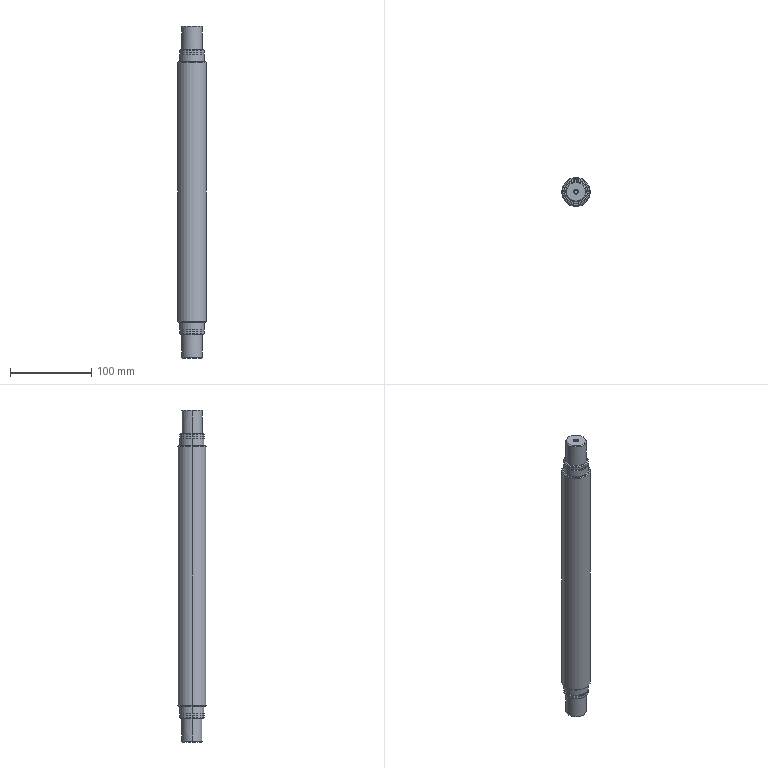Part | STEP file | Idler roller shaft | 1 solid | 50 faces | box 35 x 35 x 408 mm | volume 356727 mm3 | cylinder 22 | cone 16 | plane 12 | commonest cylinder face diameters 30 x8 4 x4 25 x4 28.6 x4 35 x2
STEP:
#1=CARTESIAN_POINT('',(-17.5,0.,334.));
#2=VERTEX_POINT('',#1);
#3=CARTESIAN_POINT('',(17.5,0.,334.));
#4=VERTEX_POINT('',#3);
#5=CARTESIAN_POINT('',(0.,0.,334.));
#6=DIRECTION('',(0.,0.,-1.));
#7=DIRECTION('',(-1.,0.,0.));
#8=AXIS2_PLACEMENT_3D('',#5,#6,#7);
#9=CIRCLE('',#8,17.5);
#10=EDGE_CURVE('',#2,#4,#9,.T.);
#11=ORIENTED_EDGE('',*,*,#10,.T.);
#12=CARTESIAN_POINT('',(17.5,0.,16.));
#13=VERTEX_POINT('',#12);
#14=CARTESIAN_POINT('',(17.5,0.,350.));
#15=DIRECTION('',(0.,0.,-1.));
#16=VECTOR('',#15,1000.);
#17=LINE('',#14,#16);
#18=EDGE_CURVE('',#4,#13,#17,.T.);
#19=ORIENTED_EDGE('',*,*,#18,.T.);
#20=CARTESIAN_POINT('',(-17.5,0.,16.));
#21=VERTEX_POINT('',#20);
#22=CARTESIAN_POINT('',(0.,0.,16.));
#23=DIRECTION('',(0.,0.,1.));
#24=DIRECTION('',(-1.,0.,0.));
#25=AXIS2_PLACEMENT_3D('',#22,#23,#24);
#26=CIRCLE('',#25,17.5);
#27=EDGE_CURVE('',#13,#21,#26,.T.);
#28=ORIENTED_EDGE('',*,*,#27,.T.);
#29=CARTESIAN_POINT('',(-17.5,0.,350.));
#30=DIRECTION('',(0.,0.,-1.));
#31=VECTOR('',#30,1000.);
#32=LINE('',#29,#31);
#33=EDGE_CURVE('',#2,#21,#32,.T.);
#34=ORIENTED_EDGE('',*,*,#33,.F.);
#35=EDGE_LOOP('',(#11,#19,#28,#34));
#36=FACE_OUTER_BOUND('',#35,.T.);
#37=CARTESIAN_POINT('',(0.,0.,350.));
#38=DIRECTION('',(0.,0.,-1.));
#39=DIRECTION('',(-1.,0.,0.));
#40=AXIS2_PLACEMENT_3D('',#37,#38,#39);
#41=CYLINDRICAL_SURFACE('',#40,17.5);
#42=ADVANCED_FACE('',(#36),#41,.T.);
#43=CARTESIAN_POINT('',(16.5,0.,15.));
#44=VERTEX_POINT('',#43);
#45=CARTESIAN_POINT('',(-16.5,0.,15.));
#46=VERTEX_POINT('',#45);
#47=CARTESIAN_POINT('',(0.,0.,15.));
#48=DIRECTION('',(0.,0.,1.));
#49=DIRECTION('',(1.,0.,0.));
#50=AXIS2_PLACEMENT_3D('',#47,#48,#49);
#51=CIRCLE('',#50,16.5);
#52=EDGE_CURVE('',#44,#46,#51,.T.);
#53=ORIENTED_EDGE('',*,*,#52,.T.);
#54=CARTESIAN_POINT('',(-17.5,0.,16.));
#55=DIRECTION('',(-0.7071,0.,0.7071));
#56=VECTOR('',#55,1000.);
#57=LINE('',#54,#56);
#58=EDGE_CURVE('',#46,#21,#57,.T.);
#59=ORIENTED_EDGE('',*,*,#58,.T.);
#60=ORIENTED_EDGE('',*,*,#27,.F.);
#61=CARTESIAN_POINT('',(17.5,0.,16.));
#62=DIRECTION('',(0.7071,0.,0.7071));
#63=VECTOR('',#62,1000.);
#64=LINE('',#61,#63);
#65=EDGE_CURVE('',#44,#13,#64,.T.);
#66=ORIENTED_EDGE('',*,*,#65,.F.);
#67=EDGE_LOOP('',(#53,#59,#60,#66));
#68=FACE_OUTER_BOUND('',#67,.T.);
#69=CARTESIAN_POINT('',(0.,0.,16.));
#70=DIRECTION('',(0.,0.,1.));
#71=DIRECTION('',(1.,0.,0.));
#72=AXIS2_PLACEMENT_3D('',#69,#70,#71);
#73=CONICAL_SURFACE('',#72,17.5,0.7854);
#74=ADVANCED_FACE('',(#68),#73,.T.);
#75=CARTESIAN_POINT('',(-16.5,0.,335.));
#76=VERTEX_POINT('',#75);
#77=CARTESIAN_POINT('',(16.5,0.,335.));
#78=VERTEX_POINT('',#77);
#79=CARTESIAN_POINT('',(0.,0.,335.));
#80=DIRECTION('',(0.,0.,-1.));
#81=DIRECTION('',(-1.,0.,0.));
#82=AXIS2_PLACEMENT_3D('',#79,#80,#81);
#83=CIRCLE('',#82,16.5);
#84=EDGE_CURVE('',#76,#78,#83,.T.);
#85=ORIENTED_EDGE('',*,*,#84,.T.);
#86=CARTESIAN_POINT('',(17.5,0.,334.));
#87=DIRECTION('',(0.7071,0.,-0.7071));
#88=VECTOR('',#87,1000.);
#89=LINE('',#86,#88);
#90=EDGE_CURVE('',#78,#4,#89,.T.);
#91=ORIENTED_EDGE('',*,*,#90,.T.);
#92=ORIENTED_EDGE('',*,*,#10,.F.);
#93=CARTESIAN_POINT('',(-17.5,0.,334.));
#94=DIRECTION('',(-0.7071,0.,-0.7071));
#95=VECTOR('',#94,1000.);
#96=LINE('',#93,#95);
#97=EDGE_CURVE('',#76,#2,#96,.T.);
#98=ORIENTED_EDGE('',*,*,#97,.F.);
#99=EDGE_LOOP('',(#85,#91,#92,#98));
#100=FACE_OUTER_BOUND('',#99,.T.);
#101=CARTESIAN_POINT('',(0.,0.,334.));
#102=DIRECTION('',(0.,0.,-1.));
#103=DIRECTION('',(-1.,0.,0.));
#104=AXIS2_PLACEMENT_3D('',#101,#102,#103);
#105=CONICAL_SURFACE('',#104,17.5,0.7854);
#106=ADVANCED_FACE('',(#100),#105,.T.);
#107=CARTESIAN_POINT('',(15.,0.,15.));
#108=VERTEX_POINT('',#107);
#109=CARTESIAN_POINT('',(-15.,0.,15.));
#110=VERTEX_POINT('',#109);
#111=CARTESIAN_POINT('',(0.,0.,15.));
#112=DIRECTION('',(0.,0.,1.));
#113=DIRECTION('',(-1.,0.,0.));
#114=AXIS2_PLACEMENT_3D('',#111,#112,#113);
#115=CIRCLE('',#114,15.);
#116=EDGE_CURVE('',#108,#110,#115,.T.);
#117=ORIENTED_EDGE('',*,*,#116,.F.);
#118=CARTESIAN_POINT('',(15.,0.,6.));
#119=VERTEX_POINT('',#118);
#120=CARTESIAN_POINT('',(15.,0.,15.));
#121=DIRECTION('',(0.,0.,-1.));
#122=VECTOR('',#121,1000.);
#123=LINE('',#120,#122);
#124=EDGE_CURVE('',#108,#119,#123,.T.);
#125=ORIENTED_EDGE('',*,*,#124,.T.);
#126=CARTESIAN_POINT('',(-15.,0.,6.));
#127=VERTEX_POINT('',#126);
#128=CARTESIAN_POINT('',(0.,0.,6.));
#129=DIRECTION('',(0.,0.,1.));
#130=DIRECTION('',(-1.,0.,0.));
#131=AXIS2_PLACEMENT_3D('',#128,#129,#130);
#132=CIRCLE('',#131,15.);
#133=EDGE_CURVE('',#119,#127,#132,.T.);
#134=ORIENTED_EDGE('',*,*,#133,.T.);
#135=CARTESIAN_POINT('',(-15.,0.,15.));
#136=DIRECTION('',(0.,0.,-1.));
#137=VECTOR('',#136,1000.);
#138=LINE('',#135,#137);
#139=EDGE_CURVE('',#110,#127,#138,.T.);
#140=ORIENTED_EDGE('',*,*,#139,.F.);
#141=EDGE_LOOP('',(#117,#125,#134,#140));
#142=FACE_OUTER_BOUND('',#141,.T.);
#143=CARTESIAN_POINT('',(0.,0.,15.));
#144=DIRECTION('',(0.,0.,-1.));
#145=DIRECTION('',(-1.,0.,0.));
#146=AXIS2_PLACEMENT_3D('',#143,#144,#145);
#147=CYLINDRICAL_SURFACE('',#146,15.);
#148=ADVANCED_FACE('',(#142),#147,.T.);
#149=CARTESIAN_POINT('',(-15.,0.,335.));
#150=VERTEX_POINT('',#149);
#151=CARTESIAN_POINT('',(15.,0.,335.));
#152=VERTEX_POINT('',#151);
#153=CARTESIAN_POINT('',(0.,0.,335.));
#154=DIRECTION('',(0.,0.,-1.));
#155=DIRECTION('',(1.,0.,0.));
#156=AXIS2_PLACEMENT_3D('',#153,#154,#155);
#157=CIRCLE('',#156,15.);
#158=EDGE_CURVE('',#150,#152,#157,.T.);
#159=ORIENTED_EDGE('',*,*,#158,.F.);
#160=CARTESIAN_POINT('',(-15.,0.,344.));
#161=VERTEX_POINT('',#160);
#162=CARTESIAN_POINT('',(-15.,0.,335.));
#163=DIRECTION('',(0.,0.,1.));
#164=VECTOR('',#163,1000.);
#165=LINE('',#162,#164);
#166=EDGE_CURVE('',#150,#161,#165,.T.);
#167=ORIENTED_EDGE('',*,*,#166,.T.);
#168=CARTESIAN_POINT('',(15.,0.,344.));
#169=VERTEX_POINT('',#168);
#170=CARTESIAN_POINT('',(0.,0.,344.));
#171=DIRECTION('',(0.,0.,-1.));
#172=DIRECTION('',(1.,0.,0.));
#173=AXIS2_PLACEMENT_3D('',#170,#171,#172);
#174=CIRCLE('',#173,15.);
#175=EDGE_CURVE('',#161,#169,#174,.T.);
#176=ORIENTED_EDGE('',*,*,#175,.T.);
#177=CARTESIAN_POINT('',(15.,0.,335.));
#178=DIRECTION('',(0.,0.,1.));
#179=VECTOR('',#178,1000.);
#180=LINE('',#177,#179);
#181=EDGE_CURVE('',#152,#169,#180,.T.);
#182=ORIENTED_EDGE('',*,*,#181,.F.);
#183=EDGE_LOOP('',(#159,#167,#176,#182));
#184=FACE_OUTER_BOUND('',#183,.T.);
#185=CARTESIAN_POINT('',(0.,0.,335.));
#186=DIRECTION('',(0.,0.,1.));
#187=DIRECTION('',(1.,0.,0.));
#188=AXIS2_PLACEMENT_3D('',#185,#186,#187);
#189=CYLINDRICAL_SURFACE('',#188,15.);
#190=ADVANCED_FACE('',(#184),#189,.T.);
#191=CARTESIAN_POINT('',(-14.3,0.,6.));
#192=VERTEX_POINT('',#191);
#193=CARTESIAN_POINT('',(14.3,0.,6.));
#194=VERTEX_POINT('',#193);
#195=CARTESIAN_POINT('',(0.,0.,6.));
#196=DIRECTION('',(0.,0.,-1.));
#197=DIRECTION('',(-1.,0.,0.));
#198=AXIS2_PLACEMENT_3D('',#195,#196,#197);
#199=CIRCLE('',#198,14.3);
#200=EDGE_CURVE('',#192,#194,#199,.T.);
#201=ORIENTED_EDGE('',*,*,#200,.T.);
#202=CARTESIAN_POINT('',(14.3,0.,4.));
#203=VERTEX_POINT('',#202);
#204=CARTESIAN_POINT('',(14.3,0.,-29.));
#205=DIRECTION('',(0.,0.,-1.));
#206=VECTOR('',#205,1000.);
#207=LINE('',#204,#206);
#208=EDGE_CURVE('',#194,#203,#207,.T.);
#209=ORIENTED_EDGE('',*,*,#208,.T.);
#210=CARTESIAN_POINT('',(-14.3,0.,4.));
#211=VERTEX_POINT('',#210);
#212=CARTESIAN_POINT('',(0.,0.,4.));
#213=DIRECTION('',(0.,0.,1.));
#214=DIRECTION('',(-1.,0.,0.));
#215=AXIS2_PLACEMENT_3D('',#212,#213,#214);
#216=CIRCLE('',#215,14.3);
#217=EDGE_CURVE('',#203,#211,#216,.T.);
#218=ORIENTED_EDGE('',*,*,#217,.T.);
#219=CARTESIAN_POINT('',(-14.3,0.,-29.));
#220=DIRECTION('',(0.,0.,-1.));
#221=VECTOR('',#220,1000.);
#222=LINE('',#219,#221);
#223=EDGE_CURVE('',#192,#211,#222,.T.);
#224=ORIENTED_EDGE('',*,*,#223,.F.);
#225=EDGE_LOOP('',(#201,#209,#218,#224));
#226=FACE_OUTER_BOUND('',#225,.T.);
#227=CARTESIAN_POINT('',(0.,0.,-29.));
#228=DIRECTION('',(0.,0.,-1.));
#229=DIRECTION('',(-1.,0.,0.));
#230=AXIS2_PLACEMENT_3D('',#227,#228,#229);
#231=CYLINDRICAL_SURFACE('',#230,14.3);
#232=ADVANCED_FACE('',(#226),#231,.T.);
#233=CARTESIAN_POINT('',(-14.3,0.,346.));
#234=VERTEX_POINT('',#233);
#235=CARTESIAN_POINT('',(14.3,0.,346.));
#236=VERTEX_POINT('',#235);
#237=CARTESIAN_POINT('',(0.,0.,346.));
#238=DIRECTION('',(0.,0.,-1.));
#239=DIRECTION('',(-1.,0.,0.));
#240=AXIS2_PLACEMENT_3D('',#237,#238,#239);
#241=CIRCLE('',#240,14.3);
#242=EDGE_CURVE('',#234,#236,#241,.T.);
#243=ORIENTED_EDGE('',*,*,#242,.T.);
#244=CARTESIAN_POINT('',(14.3,0.,344.));
#245=VERTEX_POINT('',#244);
#246=CARTESIAN_POINT('',(14.3,0.,-29.));
#247=DIRECTION('',(0.,0.,-1.));
#248=VECTOR('',#247,1000.);
#249=LINE('',#246,#248);
#250=EDGE_CURVE('',#236,#245,#249,.T.);
#251=ORIENTED_EDGE('',*,*,#250,.T.);
#252=CARTESIAN_POINT('',(-14.3,0.,344.));
#253=VERTEX_POINT('',#252);
#254=CARTESIAN_POINT('',(0.,0.,344.));
#255=DIRECTION('',(0.,0.,1.));
#256=DIRECTION('',(-1.,0.,0.));
#257=AXIS2_PLACEMENT_3D('',#254,#255,#256);
#258=CIRCLE('',#257,14.3);
#259=EDGE_CURVE('',#245,#253,#258,.T.);
#260=ORIENTED_EDGE('',*,*,#259,.T.);
#261=CARTESIAN_POINT('',(-14.3,0.,-29.));
#262=DIRECTION('',(0.,0.,-1.));
#263=VECTOR('',#262,1000.);
#264=LINE('',#261,#263);
#265=EDGE_CURVE('',#234,#253,#264,.T.);
#266=ORIENTED_EDGE('',*,*,#265,.F.);
#267=EDGE_LOOP('',(#243,#251,#260,#266));
#268=FACE_OUTER_BOUND('',#267,.T.);
#269=CARTESIAN_POINT('',(0.,0.,-29.));
#270=DIRECTION('',(0.,0.,-1.));
#271=DIRECTION('',(-1.,0.,0.));
#272=AXIS2_PLACEMENT_3D('',#269,#270,#271);
#273=CYLINDRICAL_SURFACE('',#272,14.3);
#274=ADVANCED_FACE('',(#268),#273,.T.);
#275=CARTESIAN_POINT('',(-15.,0.,4.));
#276=VERTEX_POINT('',#275);
#277=CARTESIAN_POINT('',(15.,0.,4.));
#278=VERTEX_POINT('',#277);
#279=CARTESIAN_POINT('',(0.,0.,4.));
#280=DIRECTION('',(0.,0.,-1.));
#281=DIRECTION('',(-1.,0.,0.));
#282=AXIS2_PLACEMENT_3D('',#279,#280,#281);
#283=CIRCLE('',#282,15.);
#284=EDGE_CURVE('',#276,#278,#283,.T.);
#285=ORIENTED_EDGE('',*,*,#284,.T.);
#286=CARTESIAN_POINT('',(15.,0.,1.));
#287=VERTEX_POINT('',#286);
#288=CARTESIAN_POINT('',(15.,0.,15.));
#289=DIRECTION('',(0.,0.,-1.));
#290=VECTOR('',#289,1000.);
#291=LINE('',#288,#290);
#292=EDGE_CURVE('',#278,#287,#291,.T.);
#293=ORIENTED_EDGE('',*,*,#292,.T.);
#294=CARTESIAN_POINT('',(-15.,0.,1.));
#295=VERTEX_POINT('',#294);
#296=CARTESIAN_POINT('',(0.,0.,1.));
#297=DIRECTION('',(0.,0.,1.));
#298=DIRECTION('',(-1.,0.,0.));
#299=AXIS2_PLACEMENT_3D('',#296,#297,#298);
#300=CIRCLE('',#299,15.);
#301=EDGE_CURVE('',#287,#295,#300,.T.);
#302=ORIENTED_EDGE('',*,*,#301,.T.);
#303=CARTESIAN_POINT('',(-15.,0.,15.));
#304=DIRECTION('',(0.,0.,-1.));
#305=VECTOR('',#304,1000.);
#306=LINE('',#303,#305);
#307=EDGE_CURVE('',#276,#295,#306,.T.);
#308=ORIENTED_EDGE('',*,*,#307,.F.);
#309=EDGE_LOOP('',(#285,#293,#302,#308));
#310=FACE_OUTER_BOUND('',#309,.T.);
#311=CARTESIAN_POINT('',(0.,0.,15.));
#312=DIRECTION('',(0.,0.,-1.));
#313=DIRECTION('',(-1.,0.,0.));
#314=AXIS2_PLACEMENT_3D('',#311,#312,#313);
#315=CYLINDRICAL_SURFACE('',#314,15.);
#316=ADVANCED_FACE('',(#310),#315,.T.);
#317=CARTESIAN_POINT('',(15.,0.,346.));
#318=VERTEX_POINT('',#317);
#319=CARTESIAN_POINT('',(-15.,0.,346.));
#320=VERTEX_POINT('',#319);
#321=CARTESIAN_POINT('',(0.,0.,346.));
#322=DIRECTION('',(0.,0.,1.));
#323=DIRECTION('',(1.,0.,0.));
#324=AXIS2_PLACEMENT_3D('',#321,#322,#323);
#325=CIRCLE('',#324,15.);
#326=EDGE_CURVE('',#318,#320,#325,.T.);
#327=ORIENTED_EDGE('',*,*,#326,.T.);
#328=CARTESIAN_POINT('',(-15.,0.,349.));
#329=VERTEX_POINT('',#328);
#330=CARTESIAN_POINT('',(-15.,0.,335.));
#331=DIRECTION('',(0.,0.,1.));
#332=VECTOR('',#331,1000.);
#333=LINE('',#330,#332);
#334=EDGE_CURVE('',#320,#329,#333,.T.);
#335=ORIENTED_EDGE('',*,*,#334,.T.);
#336=CARTESIAN_POINT('',(15.,0.,349.));
#337=VERTEX_POINT('',#336);
#338=CARTESIAN_POINT('',(0.,0.,349.));
#339=DIRECTION('',(0.,0.,-1.));
#340=DIRECTION('',(1.,0.,0.));
#341=AXIS2_PLACEMENT_3D('',#338,#339,#340);
#342=CIRCLE('',#341,15.);
#343=EDGE_CURVE('',#329,#337,#342,.T.);
#344=ORIENTED_EDGE('',*,*,#343,.T.);
#345=CARTESIAN_POINT('',(15.,0.,335.));
#346=DIRECTION('',(0.,0.,1.));
#347=VECTOR('',#346,1000.);
#348=LINE('',#345,#347);
#349=EDGE_CURVE('',#318,#337,#348,.T.);
#350=ORIENTED_EDGE('',*,*,#349,.F.);
#351=EDGE_LOOP('',(#327,#335,#344,#350));
#352=FACE_OUTER_BOUND('',#351,.T.);
#353=CARTESIAN_POINT('',(0.,0.,335.));
#354=DIRECTION('',(0.,0.,1.));
#355=DIRECTION('',(1.,0.,0.));
#356=AXIS2_PLACEMENT_3D('',#353,#354,#355);
#357=CYLINDRICAL_SURFACE('',#356,15.);
#358=ADVANCED_FACE('',(#352),#357,.T.);
#359=CARTESIAN_POINT('',(14.,0.,0.));
#360=VERTEX_POINT('',#359);
#361=CARTESIAN_POINT('',(-14.,0.,0.));
#362=VERTEX_POINT('',#361);
#363=CARTESIAN_POINT('',(0.,0.,0.));
#364=DIRECTION('',(0.,0.,1.));
#365=DIRECTION('',(1.,0.,0.));
#366=AXIS2_PLACEMENT_3D('',#363,#364,#365);
#367=CIRCLE('',#366,14.);
#368=EDGE_CURVE('',#360,#362,#367,.T.);
#369=ORIENTED_EDGE('',*,*,#368,.T.);
#370=CARTESIAN_POINT('',(-15.,0.,1.));
#371=DIRECTION('',(-0.7071,0.,0.7071));
#372=VECTOR('',#371,1000.);
#373=LINE('',#370,#372);
#374=EDGE_CURVE('',#362,#295,#373,.T.);
#375=ORIENTED_EDGE('',*,*,#374,.T.);
#376=ORIENTED_EDGE('',*,*,#301,.F.);
#377=CARTESIAN_POINT('',(15.,0.,1.));
#378=DIRECTION('',(0.7071,0.,0.7071));
#379=VECTOR('',#378,1000.);
#380=LINE('',#377,#379);
#381=EDGE_CURVE('',#360,#287,#380,.T.);
#382=ORIENTED_EDGE('',*,*,#381,.F.);
#383=EDGE_LOOP('',(#369,#375,#376,#382));
#384=FACE_OUTER_BOUND('',#383,.T.);
#385=CARTESIAN_POINT('',(0.,0.,1.));
#386=DIRECTION('',(0.,0.,1.));
#387=DIRECTION('',(1.,0.,0.));
#388=AXIS2_PLACEMENT_3D('',#385,#386,#387);
#389=CONICAL_SURFACE('',#388,15.,0.7854);
#390=ADVANCED_FACE('',(#384),#389,.T.);
#391=CARTESIAN_POINT('',(-14.,0.,350.));
#392=VERTEX_POINT('',#391);
#393=CARTESIAN_POINT('',(14.,0.,350.));
#394=VERTEX_POINT('',#393);
#395=CARTESIAN_POINT('',(0.,0.,350.));
#396=DIRECTION('',(0.,0.,-1.));
#397=DIRECTION('',(-1.,0.,0.));
#398=AXIS2_PLACEMENT_3D('',#395,#396,#397);
#399=CIRCLE('',#398,14.);
#400=EDGE_CURVE('',#392,#394,#399,.T.);
#401=ORIENTED_EDGE('',*,*,#400,.T.);
#402=CARTESIAN_POINT('',(15.,0.,349.));
#403=DIRECTION('',(0.7071,0.,-0.7071));
#404=VECTOR('',#403,1000.);
#405=LINE('',#402,#404);
#406=EDGE_CURVE('',#394,#337,#405,.T.);
#407=ORIENTED_EDGE('',*,*,#406,.T.);
#408=ORIENTED_EDGE('',*,*,#343,.F.);
#409=CARTESIAN_POINT('',(-15.,0.,349.));
#410=DIRECTION('',(-0.7071,0.,-0.7071));
#411=VECTOR('',#410,1000.);
#412=LINE('',#409,#411);
#413=EDGE_CURVE('',#392,#329,#412,.T.);
#414=ORIENTED_EDGE('',*,*,#413,.F.);
#415=EDGE_LOOP('',(#401,#407,#408,#414));
#416=FACE_OUTER_BOUND('',#415,.T.);
#417=CARTESIAN_POINT('',(0.,0.,349.));
#418=DIRECTION('',(0.,0.,-1.));
#419=DIRECTION('',(-1.,0.,0.));
#420=AXIS2_PLACEMENT_3D('',#417,#418,#419);
#421=CONICAL_SURFACE('',#420,15.,0.7854);
#422=ADVANCED_FACE('',(#416),#421,.T.);
#423=CARTESIAN_POINT('',(0.,12.5,-28.));
#424=VERTEX_POINT('',#423);
#425=CARTESIAN_POINT('',(-12.5,0.,-28.));
#426=VERTEX_POINT('',#425);
#427=CARTESIAN_POINT('',(0.,0.,-28.));
#428=DIRECTION('',(0.,0.,1.));
#429=DIRECTION('',(1.,0.,0.));
#430=AXIS2_PLACEMENT_3D('',#427,#428,#429);
#431=CIRCLE('',#430,12.5);
#432=EDGE_CURVE('',#424,#426,#431,.T.);
#433=ORIENTED_EDGE('',*,*,#432,.T.);
#434=CARTESIAN_POINT('',(-12.5,0.,0.));
#435=VERTEX_POINT('',#434);
#436=CARTESIAN_POINT('',(-12.5,0.,-29.));
#437=DIRECTION('',(0.,0.,1.));
#438=VECTOR('',#437,1000.);
#439=LINE('',#436,#438);
#440=EDGE_CURVE('',#426,#435,#439,.T.);
#441=ORIENTED_EDGE('',*,*,#440,.T.);
#442=CARTESIAN_POINT('',(12.5,0.,0.));
#443=VERTEX_POINT('',#442);
#444=CARTESIAN_POINT('',(0.,0.,0.));
#445=DIRECTION('',(0.,0.,-1.));
#446=DIRECTION('',(1.,0.,0.));
#447=AXIS2_PLACEMENT_3D('',#444,#445,#446);
#448=CIRCLE('',#447,12.5);
#449=EDGE_CURVE('',#435,#443,#448,.T.);
#450=ORIENTED_EDGE('',*,*,#449,.T.);
#451=CARTESIAN_POINT('',(12.5,0.,-28.));
#452=VERTEX_POINT('',#451);
#453=CARTESIAN_POINT('',(12.5,0.,-29.));
#454=DIRECTION('',(0.,0.,1.));
#455=VECTOR('',#454,1000.);
#456=LINE('',#453,#455);
#457=EDGE_CURVE('',#452,#443,#456,.T.);
#458=ORIENTED_EDGE('',*,*,#457,.F.);
#459=CARTESIAN_POINT('',(0.,0.,-28.));
#460=DIRECTION('',(0.,0.,1.));
#461=DIRECTION('',(1.,0.,0.));
#462=AXIS2_PLACEMENT_3D('',#459,#460,#461);
#463=CIRCLE('',#462,12.5);
#464=EDGE_CURVE('',#452,#424,#463,.T.);
#465=ORIENTED_EDGE('',*,*,#464,.T.);
#466=EDGE_LOOP('',(#433,#441,#450,#458,#465));
#467=FACE_OUTER_BOUND('',#466,.T.);
#468=CARTESIAN_POINT('',(0.,0.,-29.));
#469=DIRECTION('',(0.,0.,1.));
#470=DIRECTION('',(1.,0.,0.));
#471=AXIS2_PLACEMENT_3D('',#468,#469,#470);
#472=CYLINDRICAL_SURFACE('',#471,12.5);
#473=ADVANCED_FACE('',(#467),#472,.T.);
#474=CARTESIAN_POINT('',(0.,12.5,378.));
#475=VERTEX_POINT('',#474);
#476=CARTESIAN_POINT('',(12.5,0.,378.));
#477=VERTEX_POINT('',#476);
#478=CARTESIAN_POINT('',(0.,0.,378.));
#479=DIRECTION('',(0.,0.,-1.));
#480=DIRECTION('',(-1.,0.,0.));
#481=AXIS2_PLACEMENT_3D('',#478,#479,#480);
#482=CIRCLE('',#481,12.5);
#483=EDGE_CURVE('',#475,#477,#482,.T.);
#484=ORIENTED_EDGE('',*,*,#483,.T.);
#485=CARTESIAN_POINT('',(12.5,0.,350.));
#486=VERTEX_POINT('',#485);
#487=CARTESIAN_POINT('',(12.5,0.,379.));
#488=DIRECTION('',(0.,0.,-1.));
#489=VECTOR('',#488,1000.);
#490=LINE('',#487,#489);
#491=EDGE_CURVE('',#477,#486,#490,.T.);
#492=ORIENTED_EDGE('',*,*,#491,.T.);
#493=CARTESIAN_POINT('',(-12.5,0.,350.));
#494=VERTEX_POINT('',#493);
#495=CARTESIAN_POINT('',(0.,0.,350.));
#496=DIRECTION('',(0.,0.,-1.));
#497=DIRECTION('',(-1.,0.,0.));
#498=AXIS2_PLACEMENT_3D('',#495,#496,#497);
#499=CIRCLE('',#498,12.5);
#500=EDGE_CURVE('',#494,#486,#499,.T.);
#501=ORIENTED_EDGE('',*,*,#500,.F.);
#502=CARTESIAN_POINT('',(-12.5,0.,378.));
#503=VERTEX_POINT('',#502);
#504=CARTESIAN_POINT('',(-12.5,0.,379.));
#505=DIRECTION('',(0.,0.,-1.));
#506=VECTOR('',#505,1000.);
#507=LINE('',#504,#506);
#508=EDGE_CURVE('',#503,#494,#507,.T.);
#509=ORIENTED_EDGE('',*,*,#508,.F.);
#510=CARTESIAN_POINT('',(0.,0.,378.));
#511=DIRECTION('',(0.,0.,-1.));
#512=DIRECTION('',(-1.,0.,0.));
#513=AXIS2_PLACEMENT_3D('',#510,#511,#512);
#514=CIRCLE('',#513,12.5);
#515=EDGE_CURVE('',#503,#475,#514,.T.);
#516=ORIENTED_EDGE('',*,*,#515,.T.);
#517=EDGE_LOOP('',(#484,#492,#501,#509,#516));
#518=FACE_OUTER_BOUND('',#517,.T.);
#519=CARTESIAN_POINT('',(0.,0.,379.));
#520=DIRECTION('',(0.,0.,-1.));
#521=DIRECTION('',(-1.,0.,0.));
#522=AXIS2_PLACEMENT_3D('',#519,#520,#521);
#523=CYLINDRICAL_SURFACE('',#522,12.5);
#524=ADVANCED_FACE('',(#518),#523,.T.);
#525=CARTESIAN_POINT('',(0.,-11.5,-29.));
#526=VERTEX_POINT('',#525);
#527=CARTESIAN_POINT('',(0.,11.5,-29.));
#528=VERTEX_POINT('',#527);
#529=CARTESIAN_POINT('',(0.,0.,-29.));
#530=DIRECTION('',(0.,0.,1.));
#531=DIRECTION('',(0.,-1.,0.));
#532=AXIS2_PLACEMENT_3D('',#529,#530,#531);
#533=CIRCLE('',#532,11.5);
#534=EDGE_CURVE('',#526,#528,#533,.T.);
#535=ORIENTED_EDGE('',*,*,#534,.T.);
#536=CARTESIAN_POINT('',(0.,12.5,-28.));
#537=DIRECTION('',(0.,0.7071,0.7071));
#538=VECTOR('',#537,1000.);
#539=LINE('',#536,#538);
#540=EDGE_CURVE('',#528,#424,#539,.T.);
#541=ORIENTED_EDGE('',*,*,#540,.T.);
#542=ORIENTED_EDGE('',*,*,#464,.F.);
#543=CARTESIAN_POINT('',(0.,-12.5,-28.));
#544=VERTEX_POINT('',#543);
#545=CARTESIAN_POINT('',(0.,0.,-28.));
#546=DIRECTION('',(0.,0.,1.));
#547=DIRECTION('',(1.,0.,0.));
#548=AXIS2_PLACEMENT_3D('',#545,#546,#547);
#549=CIRCLE('',#548,12.5);
#550=EDGE_CURVE('',#544,#452,#549,.T.);
#551=ORIENTED_EDGE('',*,*,#550,.F.);
#552=CARTESIAN_POINT('',(0.,-12.5,-28.));
#553=DIRECTION('',(0.,-0.7071,0.7071));
#554=VECTOR('',#553,1000.);
#555=LINE('',#552,#554);
#556=EDGE_CURVE('',#526,#544,#555,.T.);
#557=ORIENTED_EDGE('',*,*,#556,.F.);
#558=EDGE_LOOP('',(#535,#541,#542,#551,#557));
#559=FACE_OUTER_BOUND('',#558,.T.);
#560=CARTESIAN_POINT('',(0.,0.,-28.));
#561=DIRECTION('',(0.,0.,1.));
#562=DIRECTION('',(0.,-1.,0.));
#563=AXIS2_PLACEMENT_3D('',#560,#561,#562);
#564=CONICAL_SURFACE('',#563,12.5,0.7854);
#565=ADVANCED_FACE('',(#559),#564,.T.);
#566=CARTESIAN_POINT('',(0.,11.5,379.));
#567=VERTEX_POINT('',#566);
#568=CARTESIAN_POINT('',(0.,-11.5,379.));
#569=VERTEX_POINT('',#568);
#570=CARTESIAN_POINT('',(0.,0.,379.));
#571=DIRECTION('',(0.,0.,-1.));
#572=DIRECTION('',(0.,1.,0.));
#573=AXIS2_PLACEMENT_3D('',#570,#571,#572);
#574=CIRCLE('',#573,11.5);
#575=EDGE_CURVE('',#567,#569,#574,.T.);
#576=ORIENTED_EDGE('',*,*,#575,.T.);
#577=CARTESIAN_POINT('',(0.,-12.5,378.));
#578=VERTEX_POINT('',#577);
#579=CARTESIAN_POINT('',(0.,-12.5,378.));
#580=DIRECTION('',(0.,-0.7071,-0.7071));
#581=VECTOR('',#580,1000.);
#582=LINE('',#579,#581);
#583=EDGE_CURVE('',#569,#578,#582,.T.);
#584=ORIENTED_EDGE('',*,*,#583,.T.);
#585=CARTESIAN_POINT('',(0.,0.,378.));
#586=DIRECTION('',(0.,0.,-1.));
#587=DIRECTION('',(-1.,0.,0.));
#588=AXIS2_PLACEMENT_3D('',#585,#586,#587);
#589=CIRCLE('',#588,12.5);
#590=EDGE_CURVE('',#477,#578,#589,.T.);
#591=ORIENTED_EDGE('',*,*,#590,.F.);
#592=ORIENTED_EDGE('',*,*,#483,.F.);
#593=CARTESIAN_POINT('',(0.,12.5,378.));
#594=DIRECTION('',(0.,0.7071,-0.7071));
#595=VECTOR('',#594,1000.);
#596=LINE('',#593,#595);
#597=EDGE_CURVE('',#567,#475,#596,.T.);
#598=ORIENTED_EDGE('',*,*,#597,.F.);
#599=EDGE_LOOP('',(#576,#584,#591,#592,#598));
#600=FACE_OUTER_BOUND('',#599,.T.);
#601=CARTESIAN_POINT('',(0.,0.,378.));
#602=DIRECTION('',(0.,0.,-1.));
#603=DIRECTION('',(0.,1.,0.));
#604=AXIS2_PLACEMENT_3D('',#601,#602,#603);
#605=CONICAL_SURFACE('',#604,12.5,0.7854);
#606=ADVANCED_FACE('',(#600),#605,.T.);
#607=CARTESIAN_POINT('',(0.,-2.,-28.));
#608=VERTEX_POINT('',#607);
#609=CARTESIAN_POINT('',(-2.,0.,-28.));
#610=VERTEX_POINT('',#609);
#611=CARTESIAN_POINT('',(0.,0.,-28.));
#612=DIRECTION('',(0.,0.,-1.));
#613=DIRECTION('',(-1.,0.,0.));
#614=AXIS2_PLACEMENT_3D('',#611,#612,#613);
#615=CIRCLE('',#614,2.);
#616=EDGE_CURVE('',#608,#610,#615,.T.);
#617=ORIENTED_EDGE('',*,*,#616,.F.);
#618=CARTESIAN_POINT('',(0.,-3.,-29.));
#619=VERTEX_POINT('',#618);
#620=CARTESIAN_POINT('',(0.,-3.,-29.));
#621=DIRECTION('',(0.,-0.7071,-0.7071));
#622=VECTOR('',#621,1000.);
#623=LINE('',#620,#622);
#624=EDGE_CURVE('',#608,#619,#623,.T.);
#625=ORIENTED_EDGE('',*,*,#624,.T.);
#626=CARTESIAN_POINT('',(0.,3.,-29.));
#627=VERTEX_POINT('',#626);
#628=CARTESIAN_POINT('',(0.,0.,-29.));
#629=DIRECTION('',(0.,0.,1.));
#630=DIRECTION('',(0.,1.,0.));
#631=AXIS2_PLACEMENT_3D('',#628,#629,#630);
#632=CIRCLE('',#631,3.);
#633=EDGE_CURVE('',#627,#619,#632,.T.);
#634=ORIENTED_EDGE('',*,*,#633,.F.);
#635=CARTESIAN_POINT('',(0.,2.,-28.));
#636=VERTEX_POINT('',#635);
#637=CARTESIAN_POINT('',(0.,3.,-29.));
#638=DIRECTION('',(0.,0.7071,-0.7071));
#639=VECTOR('',#638,1000.);
#640=LINE('',#637,#639);
#641=EDGE_CURVE('',#636,#627,#640,.T.);
#642=ORIENTED_EDGE('',*,*,#641,.F.);
#643=CARTESIAN_POINT('',(0.,0.,-28.));
#644=DIRECTION('',(0.,0.,-1.));
#645=DIRECTION('',(-1.,0.,0.));
#646=AXIS2_PLACEMENT_3D('',#643,#644,#645);
#647=CIRCLE('',#646,2.);
#648=EDGE_CURVE('',#610,#636,#647,.T.);
#649=ORIENTED_EDGE('',*,*,#648,.F.);
#650=EDGE_LOOP('',(#617,#625,#634,#642,#649));
#651=FACE_OUTER_BOUND('',#650,.T.);
#652=CARTESIAN_POINT('',(0.,0.,-29.));
#653=DIRECTION('',(0.,0.,-1.));
#654=DIRECTION('',(0.,1.,0.));
#655=AXIS2_PLACEMENT_3D('',#652,#653,#654);
#656=CONICAL_SURFACE('',#655,3.,0.7854);
#657=ADVANCED_FACE('',(#651),#656,.F.);
#658=CARTESIAN_POINT('',(-2.,0.,378.));
#659=VERTEX_POINT('',#658);
#660=CARTESIAN_POINT('',(2.,0.,378.));
#661=VERTEX_POINT('',#660);
#662=CARTESIAN_POINT('',(0.,0.,378.));
#663=DIRECTION('',(0.,0.,1.));
#664=DIRECTION('',(1.,0.,0.));
#665=AXIS2_PLACEMENT_3D('',#662,#663,#664);
#666=CIRCLE('',#665,2.);
#667=EDGE_CURVE('',#659,#661,#666,.T.);
#668=ORIENTED_EDGE('',*,*,#667,.F.);
#669=CARTESIAN_POINT('',(-3.,0.,379.));
#670=VERTEX_POINT('',#669);
#671=CARTESIAN_POINT('',(-3.,0.,379.));
#672=DIRECTION('',(-0.7071,0.,0.7071));
#673=VECTOR('',#672,1000.);
#674=LINE('',#671,#673);
#675=EDGE_CURVE('',#659,#670,#674,.T.);
#676=ORIENTED_EDGE('',*,*,#675,.T.);
#677=CARTESIAN_POINT('',(3.,0.,379.));
#678=VERTEX_POINT('',#677);
#679=CARTESIAN_POINT('',(0.,0.,379.));
#680=DIRECTION('',(0.,0.,-1.));
#681=DIRECTION('',(1.,0.,0.));
#682=AXIS2_PLACEMENT_3D('',#679,#680,#681);
#683=CIRCLE('',#682,3.);
#684=EDGE_CURVE('',#678,#670,#683,.T.);
#685=ORIENTED_EDGE('',*,*,#684,.F.);
#686=CARTESIAN_POINT('',(3.,0.,379.));
#687=DIRECTION('',(0.7071,0.,0.7071));
#688=VECTOR('',#687,1000.);
#689=LINE('',#686,#688);
#690=EDGE_CURVE('',#661,#678,#689,.T.);
#691=ORIENTED_EDGE('',*,*,#690,.F.);
#692=EDGE_LOOP('',(#668,#676,#685,#691));
#693=FACE_OUTER_BOUND('',#692,.T.);
#694=CARTESIAN_POINT('',(0.,0.,379.));
#695=DIRECTION('',(0.,0.,1.));
#696=DIRECTION('',(1.,0.,0.));
#697=AXIS2_PLACEMENT_3D('',#694,#695,#696);
#698=CONICAL_SURFACE('',#697,3.,0.7854);
#699=ADVANCED_FACE('',(#693),#698,.F.);
#700=CARTESIAN_POINT('',(2.,0.,-18.));
#701=VERTEX_POINT('',#700);
#702=CARTESIAN_POINT('',(-2.,0.,-18.));
#703=VERTEX_POINT('',#702);
#704=CARTESIAN_POINT('',(0.,0.,-18.));
#705=DIRECTION('',(0.,0.,-1.));
#706=DIRECTION('',(-1.,0.,0.));
#707=AXIS2_PLACEMENT_3D('',#704,#705,#706);
#708=CIRCLE('',#707,2.);
#709=EDGE_CURVE('',#701,#703,#708,.T.);
#710=ORIENTED_EDGE('',*,*,#709,.F.);
#711=CARTESIAN_POINT('',(2.,0.,-28.));
#712=VERTEX_POINT('',#711);
#713=CARTESIAN_POINT('',(2.,0.,-18.));
#714=DIRECTION('',(0.,0.,-1.));
#715=VECTOR('',#714,1000.);
#716=LINE('',#713,#715);
#717=EDGE_CURVE('',#701,#712,#716,.T.);
#718=ORIENTED_EDGE('',*,*,#717,.T.);
#719=CARTESIAN_POINT('',(0.,0.,-28.));
#720=DIRECTION('',(0.,0.,-1.));
#721=DIRECTION('',(-1.,0.,0.));
#722=AXIS2_PLACEMENT_3D('',#719,#720,#721);
#723=CIRCLE('',#722,2.);
#724=EDGE_CURVE('',#712,#608,#723,.T.);
#725=ORIENTED_EDGE('',*,*,#724,.T.);
#726=ORIENTED_EDGE('',*,*,#616,.T.);
#727=CARTESIAN_POINT('',(-2.,0.,-18.));
#728=DIRECTION('',(0.,0.,-1.));
#729=VECTOR('',#728,1000.);
#730=LINE('',#727,#729);
#731=EDGE_CURVE('',#703,#610,#730,.T.);
#732=ORIENTED_EDGE('',*,*,#731,.F.);
#733=EDGE_LOOP('',(#710,#718,#725,#726,#732));
#734=FACE_OUTER_BOUND('',#733,.T.);
#735=CARTESIAN_POINT('',(0.,0.,-18.));
#736=DIRECTION('',(0.,0.,-1.));
#737=DIRECTION('',(-1.,0.,0.));
#738=AXIS2_PLACEMENT_3D('',#735,#736,#737);
#739=CYLINDRICAL_SURFACE('',#738,2.);
#740=ADVANCED_FACE('',(#734),#739,.F.);
#741=CARTESIAN_POINT('',(-2.,0.,368.));
#742=VERTEX_POINT('',#741);
#743=CARTESIAN_POINT('',(2.,0.,368.));
#744=VERTEX_POINT('',#743);
#745=CARTESIAN_POINT('',(0.,0.,368.));
#746=DIRECTION('',(0.,0.,1.));
#747=DIRECTION('',(1.,0.,0.));
#748=AXIS2_PLACEMENT_3D('',#745,#746,#747);
#749=CIRCLE('',#748,2.);
#750=EDGE_CURVE('',#742,#744,#749,.T.);
#751=ORIENTED_EDGE('',*,*,#750,.F.);
#752=CARTESIAN_POINT('',(-2.,0.,368.));
#753=DIRECTION('',(0.,0.,1.));
#754=VECTOR('',#753,1000.);
#755=LINE('',#752,#754);
#756=EDGE_CURVE('',#742,#659,#755,.T.);
#757=ORIENTED_EDGE('',*,*,#756,.T.);
#758=ORIENTED_EDGE('',*,*,#667,.T.);
#759=CARTESIAN_POINT('',(2.,0.,368.));
#760=DIRECTION('',(0.,0.,1.));
#761=VECTOR('',#760,1000.);
#762=LINE('',#759,#761);
#763=EDGE_CURVE('',#744,#661,#762,.T.);
#764=ORIENTED_EDGE('',*,*,#763,.F.);
#765=EDGE_LOOP('',(#751,#757,#758,#764));
#766=FACE_OUTER_BOUND('',#765,.T.);
#767=CARTESIAN_POINT('',(0.,0.,368.));
#768=DIRECTION('',(0.,0.,1.));
#769=DIRECTION('',(1.,0.,0.));
#770=AXIS2_PLACEMENT_3D('',#767,#768,#769);
#771=CYLINDRICAL_SURFACE('',#770,2.);
#772=ADVANCED_FACE('',(#766),#771,.F.);
#773=ORIENTED_EDGE('',*,*,#18,.F.);
#774=CARTESIAN_POINT('',(0.,0.,334.));
#775=DIRECTION('',(0.,0.,-1.));
#776=DIRECTION('',(-1.,0.,0.));
#777=AXIS2_PLACEMENT_3D('',#774,#775,#776);
#778=CIRCLE('',#777,17.5);
#779=EDGE_CURVE('',#4,#2,#778,.T.);
#780=ORIENTED_EDGE('',*,*,#779,.T.);
#781=ORIENTED_EDGE('',*,*,#33,.T.);
#782=CARTESIAN_POINT('',(0.,0.,16.));
#783=DIRECTION('',(0.,0.,1.));
#784=DIRECTION('',(-1.,0.,0.));
#785=AXIS2_PLACEMENT_3D('',#782,#783,#784);
#786=CIRCLE('',#785,17.5);
#787=EDGE_CURVE('',#21,#13,#786,.T.);
#788=ORIENTED_EDGE('',*,*,#787,.T.);
#789=EDGE_LOOP('',(#773,#780,#781,#788));
#790=FACE_OUTER_BOUND('',#789,.T.);
#791=CARTESIAN_POINT('',(0.,0.,350.));
#792=DIRECTION('',(0.,0.,-1.));
#793=DIRECTION('',(-1.,0.,0.));
#794=AXIS2_PLACEMENT_3D('',#791,#792,#793);
#795=CYLINDRICAL_SURFACE('',#794,17.5);
#796=ADVANCED_FACE('',(#790),#795,.T.);
#797=ORIENTED_EDGE('',*,*,#58,.F.);
#798=CARTESIAN_POINT('',(0.,0.,15.));
#799=DIRECTION('',(0.,0.,1.));
#800=DIRECTION('',(1.,0.,0.));
#801=AXIS2_PLACEMENT_3D('',#798,#799,#800);
#802=CIRCLE('',#801,16.5);
#803=EDGE_CURVE('',#46,#44,#802,.T.);
#804=ORIENTED_EDGE('',*,*,#803,.T.);
#805=ORIENTED_EDGE('',*,*,#65,.T.);
#806=ORIENTED_EDGE('',*,*,#787,.F.);
#807=EDGE_LOOP('',(#797,#804,#805,#806));
#808=FACE_OUTER_BOUND('',#807,.T.);
#809=CARTESIAN_POINT('',(0.,0.,16.));
#810=DIRECTION('',(0.,0.,1.));
#811=DIRECTION('',(1.,0.,0.));
#812=AXIS2_PLACEMENT_3D('',#809,#810,#811);
#813=CONICAL_SURFACE('',#812,17.5,0.7854);
#814=ADVANCED_FACE('',(#808),#813,.T.);
#815=ORIENTED_EDGE('',*,*,#90,.F.);
#816=CARTESIAN_POINT('',(0.,0.,335.));
#817=DIRECTION('',(0.,0.,-1.));
#818=DIRECTION('',(-1.,0.,0.));
#819=AXIS2_PLACEMENT_3D('',#816,#817,#818);
#820=CIRCLE('',#819,16.5);
#821=EDGE_CURVE('',#78,#76,#820,.T.);
#822=ORIENTED_EDGE('',*,*,#821,.T.);
#823=ORIENTED_EDGE('',*,*,#97,.T.);
#824=ORIENTED_EDGE('',*,*,#779,.F.);
#825=EDGE_LOOP('',(#815,#822,#823,#824));
#826=FACE_OUTER_BOUND('',#825,.T.);
#827=CARTESIAN_POINT('',(0.,0.,334.));
#828=DIRECTION('',(0.,0.,-1.));
#829=DIRECTION('',(-1.,0.,0.));
#830=AXIS2_PLACEMENT_3D('',#827,#828,#829);
#831=CONICAL_SURFACE('',#830,17.5,0.7854);
#832=ADVANCED_FACE('',(#826),#831,.T.);
#833=CARTESIAN_POINT('',(0.,0.,15.));
#834=DIRECTION('',(0.,0.,1.));
#835=DIRECTION('',(-1.,0.,0.));
#836=AXIS2_PLACEMENT_3D('',#833,#834,#835);
#837=CIRCLE('',#836,15.);
#838=EDGE_CURVE('',#110,#108,#837,.T.);
#839=ORIENTED_EDGE('',*,*,#838,.T.);
#840=ORIENTED_EDGE('',*,*,#116,.T.);
#841=EDGE_LOOP('',(#839,#840));
#842=FACE_BOUND('',#841,.T.);
#843=ORIENTED_EDGE('',*,*,#52,.F.);
#844=ORIENTED_EDGE('',*,*,#803,.F.);
#845=EDGE_LOOP('',(#843,#844));
#846=FACE_OUTER_BOUND('',#845,.T.);
#847=CARTESIAN_POINT('',(0.,0.,15.));
#848=DIRECTION('',(0.,0.,-1.));
#849=DIRECTION('',(-1.,0.,0.));
#850=AXIS2_PLACEMENT_3D('',#847,#848,#849);
#851=PLANE('',#850);
#852=ADVANCED_FACE('',(#842,#846),#851,.T.);
#853=CARTESIAN_POINT('',(0.,0.,335.));
#854=DIRECTION('',(0.,0.,-1.));
#855=DIRECTION('',(1.,0.,0.));
#856=AXIS2_PLACEMENT_3D('',#853,#854,#855);
#857=CIRCLE('',#856,15.);
#858=EDGE_CURVE('',#152,#150,#857,.T.);
#859=ORIENTED_EDGE('',*,*,#858,.T.);
#860=ORIENTED_EDGE('',*,*,#158,.T.);
#861=EDGE_LOOP('',(#859,#860));
#862=FACE_BOUND('',#861,.T.);
#863=ORIENTED_EDGE('',*,*,#84,.F.);
#864=ORIENTED_EDGE('',*,*,#821,.F.);
#865=EDGE_LOOP('',(#863,#864));
#866=FACE_OUTER_BOUND('',#865,.T.);
#867=CARTESIAN_POINT('',(0.,0.,335.));
#868=DIRECTION('',(0.,0.,1.));
#869=DIRECTION('',(1.,0.,0.));
#870=AXIS2_PLACEMENT_3D('',#867,#868,#869);
#871=PLANE('',#870);
#872=ADVANCED_FACE('',(#862,#866),#871,.T.);
#873=ORIENTED_EDGE('',*,*,#124,.F.);
#874=ORIENTED_EDGE('',*,*,#838,.F.);
#875=ORIENTED_EDGE('',*,*,#139,.T.);
#876=CARTESIAN_POINT('',(0.,0.,6.));
#877=DIRECTION('',(0.,0.,1.));
#878=DIRECTION('',(-1.,0.,0.));
#879=AXIS2_PLACEMENT_3D('',#876,#877,#878);
#880=CIRCLE('',#879,15.);
#881=EDGE_CURVE('',#127,#119,#880,.T.);
#882=ORIENTED_EDGE('',*,*,#881,.T.);
#883=EDGE_LOOP('',(#873,#874,#875,#882));
#884=FACE_OUTER_BOUND('',#883,.T.);
#885=CARTESIAN_POINT('',(0.,0.,15.));
#886=DIRECTION('',(0.,0.,-1.));
#887=DIRECTION('',(-1.,0.,0.));
#888=AXIS2_PLACEMENT_3D('',#885,#886,#887);
#889=CYLINDRICAL_SURFACE('',#888,15.);
#890=ADVANCED_FACE('',(#884),#889,.T.);
#891=ORIENTED_EDGE('',*,*,#166,.F.);
#892=ORIENTED_EDGE('',*,*,#858,.F.);
#893=ORIENTED_EDGE('',*,*,#181,.T.);
#894=CARTESIAN_POINT('',(0.,0.,344.));
#895=DIRECTION('',(0.,0.,-1.));
#896=DIRECTION('',(1.,0.,0.));
#897=AXIS2_PLACEMENT_3D('',#894,#895,#896);
#898=CIRCLE('',#897,15.);
#899=EDGE_CURVE('',#169,#161,#898,.T.);
#900=ORIENTED_EDGE('',*,*,#899,.T.);
#901=EDGE_LOOP('',(#891,#892,#893,#900));
#902=FACE_OUTER_BOUND('',#901,.T.);
#903=CARTESIAN_POINT('',(0.,0.,335.));
#904=DIRECTION('',(0.,0.,1.));
#905=DIRECTION('',(1.,0.,0.));
#906=AXIS2_PLACEMENT_3D('',#903,#904,#905);
#907=CYLINDRICAL_SURFACE('',#906,15.);
#908=ADVANCED_FACE('',(#902),#907,.T.);
#909=ORIENTED_EDGE('',*,*,#200,.F.);
#910=CARTESIAN_POINT('',(0.,0.,6.));
#911=DIRECTION('',(0.,0.,-1.));
#912=DIRECTION('',(-1.,0.,0.));
#913=AXIS2_PLACEMENT_3D('',#910,#911,#912);
#914=CIRCLE('',#913,14.3);
#915=EDGE_CURVE('',#194,#192,#914,.T.);
#916=ORIENTED_EDGE('',*,*,#915,.F.);
#917=EDGE_LOOP('',(#909,#916));
#918=FACE_BOUND('',#917,.T.);
#919=ORIENTED_EDGE('',*,*,#881,.F.);
#920=ORIENTED_EDGE('',*,*,#133,.F.);
#921=EDGE_LOOP('',(#919,#920));
#922=FACE_OUTER_BOUND('',#921,.T.);
#923=CARTESIAN_POINT('',(-19.3,0.,6.));
#924=DIRECTION('',(0.,0.,1.));
#925=DIRECTION('',(1.,0.,0.));
#926=AXIS2_PLACEMENT_3D('',#923,#924,#925);
#927=PLANE('',#926);
#928=ADVANCED_FACE('',(#918,#922),#927,.F.);
#929=CARTESIAN_POINT('',(0.,0.,344.));
#930=DIRECTION('',(0.,0.,1.));
#931=DIRECTION('',(-1.,0.,0.));
#932=AXIS2_PLACEMENT_3D('',#929,#930,#931);
#933=CIRCLE('',#932,14.3);
#934=EDGE_CURVE('',#253,#245,#933,.T.);
#935=ORIENTED_EDGE('',*,*,#934,.F.);
#936=ORIENTED_EDGE('',*,*,#259,.F.);
#937=EDGE_LOOP('',(#935,#936));
#938=FACE_BOUND('',#937,.T.);
#939=ORIENTED_EDGE('',*,*,#899,.F.);
#940=ORIENTED_EDGE('',*,*,#175,.F.);
#941=EDGE_LOOP('',(#939,#940));
#942=FACE_OUTER_BOUND('',#941,.T.);
#943=CARTESIAN_POINT('',(-23.3,0.,344.));
#944=DIRECTION('',(0.,0.,-1.));
#945=DIRECTION('',(-1.,0.,0.));
#946=AXIS2_PLACEMENT_3D('',#943,#944,#945);
#947=PLANE('',#946);
#948=ADVANCED_FACE('',(#938,#942),#947,.F.);
#949=ORIENTED_EDGE('',*,*,#208,.F.);
#950=ORIENTED_EDGE('',*,*,#915,.T.);
#951=ORIENTED_EDGE('',*,*,#223,.T.);
#952=CARTESIAN_POINT('',(0.,0.,4.));
#953=DIRECTION('',(0.,0.,1.));
#954=DIRECTION('',(-1.,0.,0.));
#955=AXIS2_PLACEMENT_3D('',#952,#953,#954);
#956=CIRCLE('',#955,14.3);
#957=EDGE_CURVE('',#211,#203,#956,.T.);
#958=ORIENTED_EDGE('',*,*,#957,.T.);
#959=EDGE_LOOP('',(#949,#950,#951,#958));
#960=FACE_OUTER_BOUND('',#959,.T.);
#961=CARTESIAN_POINT('',(0.,0.,-29.));
#962=DIRECTION('',(0.,0.,-1.));
#963=DIRECTION('',(-1.,0.,0.));
#964=AXIS2_PLACEMENT_3D('',#961,#962,#963);
#965=CYLINDRICAL_SURFACE('',#964,14.3);
#966=ADVANCED_FACE('',(#960),#965,.T.);
#967=ORIENTED_EDGE('',*,*,#250,.F.);
#968=CARTESIAN_POINT('',(0.,0.,346.));
#969=DIRECTION('',(0.,0.,-1.));
#970=DIRECTION('',(-1.,0.,0.));
#971=AXIS2_PLACEMENT_3D('',#968,#969,#970);
#972=CIRCLE('',#971,14.3);
#973=EDGE_CURVE('',#236,#234,#972,.T.);
#974=ORIENTED_EDGE('',*,*,#973,.T.);
#975=ORIENTED_EDGE('',*,*,#265,.T.);
#976=ORIENTED_EDGE('',*,*,#934,.T.);
#977=EDGE_LOOP('',(#967,#974,#975,#976));
#978=FACE_OUTER_BOUND('',#977,.T.);
#979=CARTESIAN_POINT('',(0.,0.,-29.));
#980=DIRECTION('',(0.,0.,-1.));
#981=DIRECTION('',(-1.,0.,0.));
#982=AXIS2_PLACEMENT_3D('',#979,#980,#981);
#983=CYLINDRICAL_SURFACE('',#982,14.3);
#984=ADVANCED_FACE('',(#978),#983,.T.);
#985=ORIENTED_EDGE('',*,*,#957,.F.);
#986=ORIENTED_EDGE('',*,*,#217,.F.);
#987=EDGE_LOOP('',(#985,#986));
#988=FACE_BOUND('',#987,.T.);
#989=ORIENTED_EDGE('',*,*,#284,.F.);
#990=CARTESIAN_POINT('',(0.,0.,4.));
#991=DIRECTION('',(0.,0.,-1.));
#992=DIRECTION('',(-1.,0.,0.));
#993=AXIS2_PLACEMENT_3D('',#990,#991,#992);
#994=CIRCLE('',#993,15.);
#995=EDGE_CURVE('',#278,#276,#994,.T.);
#996=ORIENTED_EDGE('',*,*,#995,.F.);
#997=EDGE_LOOP('',(#989,#996));
#998=FACE_OUTER_BOUND('',#997,.T.);
#999=CARTESIAN_POINT('',(-19.3,0.,4.));
#1000=DIRECTION('',(0.,0.,-1.));
#1001=DIRECTION('',(-1.,0.,0.));
#1002=AXIS2_PLACEMENT_3D('',#999,#1000,#1001);
#1003=PLANE('',#1002);
#1004=ADVANCED_FACE('',(#988,#998),#1003,.F.);
#1005=ORIENTED_EDGE('',*,*,#242,.F.);
#1006=ORIENTED_EDGE('',*,*,#973,.F.);
#1007=EDGE_LOOP('',(#1005,#1006));
#1008=FACE_BOUND('',#1007,.T.);
#1009=ORIENTED_EDGE('',*,*,#326,.F.);
#1010=CARTESIAN_POINT('',(0.,0.,346.));
#1011=DIRECTION('',(0.,0.,1.));
#1012=DIRECTION('',(1.,0.,0.));
#1013=AXIS2_PLACEMENT_3D('',#1010,#1011,#1012);
#1014=CIRCLE('',#1013,15.);
#1015=EDGE_CURVE('',#320,#318,#1014,.T.);
#1016=ORIENTED_EDGE('',*,*,#1015,.F.);
#1017=EDGE_LOOP('',(#1009,#1016));
#1018=FACE_OUTER_BOUND('',#1017,.T.);
#1019=CARTESIAN_POINT('',(-23.3,0.,346.));
#1020=DIRECTION('',(0.,0.,1.));
#1021=DIRECTION('',(1.,0.,0.));
#1022=AXIS2_PLACEMENT_3D('',#1019,#1020,#1021);
#1023=PLANE('',#1022);
#1024=ADVANCED_FACE('',(#1008,#1018),#1023,.F.);
#1025=ORIENTED_EDGE('',*,*,#292,.F.);
#1026=ORIENTED_EDGE('',*,*,#995,.T.);
#1027=ORIENTED_EDGE('',*,*,#307,.T.);
#1028=CARTESIAN_POINT('',(0.,0.,1.));
#1029=DIRECTION('',(0.,0.,1.));
#1030=DIRECTION('',(-1.,0.,0.));
#1031=AXIS2_PLACEMENT_3D('',#1028,#1029,#1030);
#1032=CIRCLE('',#1031,15.);
#1033=EDGE_CURVE('',#295,#287,#1032,.T.);
#1034=ORIENTED_EDGE('',*,*,#1033,.T.);
#1035=EDGE_LOOP('',(#1025,#1026,#1027,#1034));
#1036=FACE_OUTER_BOUND('',#1035,.T.);
#1037=CARTESIAN_POINT('',(0.,0.,15.));
#1038=DIRECTION('',(0.,0.,-1.));
#1039=DIRECTION('',(-1.,0.,0.));
#1040=AXIS2_PLACEMENT_3D('',#1037,#1038,#1039);
#1041=CYLINDRICAL_SURFACE('',#1040,15.);
#1042=ADVANCED_FACE('',(#1036),#1041,.T.);
#1043=ORIENTED_EDGE('',*,*,#334,.F.);
#1044=ORIENTED_EDGE('',*,*,#1015,.T.);
#1045=ORIENTED_EDGE('',*,*,#349,.T.);
#1046=CARTESIAN_POINT('',(0.,0.,349.));
#1047=DIRECTION('',(0.,0.,-1.));
#1048=DIRECTION('',(1.,0.,0.));
#1049=AXIS2_PLACEMENT_3D('',#1046,#1047,#1048);
#1050=CIRCLE('',#1049,15.);
#1051=EDGE_CURVE('',#337,#329,#1050,.T.);
#1052=ORIENTED_EDGE('',*,*,#1051,.T.);
#1053=EDGE_LOOP('',(#1043,#1044,#1045,#1052));
#1054=FACE_OUTER_BOUND('',#1053,.T.);
#1055=CARTESIAN_POINT('',(0.,0.,335.));
#1056=DIRECTION('',(0.,0.,1.));
#1057=DIRECTION('',(1.,0.,0.));
#1058=AXIS2_PLACEMENT_3D('',#1055,#1056,#1057);
#1059=CYLINDRICAL_SURFACE('',#1058,15.);
#1060=ADVANCED_FACE('',(#1054),#1059,.T.);
#1061=ORIENTED_EDGE('',*,*,#374,.F.);
#1062=CARTESIAN_POINT('',(0.,0.,0.));
#1063=DIRECTION('',(0.,0.,1.));
#1064=DIRECTION('',(1.,0.,0.));
#1065=AXIS2_PLACEMENT_3D('',#1062,#1063,#1064);
#1066=CIRCLE('',#1065,14.);
#1067=EDGE_CURVE('',#362,#360,#1066,.T.);
#1068=ORIENTED_EDGE('',*,*,#1067,.T.);
#1069=ORIENTED_EDGE('',*,*,#381,.T.);
#1070=ORIENTED_EDGE('',*,*,#1033,.F.);
#1071=EDGE_LOOP('',(#1061,#1068,#1069,#1070));
#1072=FACE_OUTER_BOUND('',#1071,.T.);
#1073=CARTESIAN_POINT('',(0.,0.,1.));
#1074=DIRECTION('',(0.,0.,1.));
#1075=DIRECTION('',(1.,0.,0.));
#1076=AXIS2_PLACEMENT_3D('',#1073,#1074,#1075);
#1077=CONICAL_SURFACE('',#1076,15.,0.7854);
#1078=ADVANCED_FACE('',(#1072),#1077,.T.);
#1079=ORIENTED_EDGE('',*,*,#406,.F.);
#1080=CARTESIAN_POINT('',(0.,0.,350.));
#1081=DIRECTION('',(0.,0.,-1.));
#1082=DIRECTION('',(-1.,0.,0.));
#1083=AXIS2_PLACEMENT_3D('',#1080,#1081,#1082);
#1084=CIRCLE('',#1083,14.);
#1085=EDGE_CURVE('',#394,#392,#1084,.T.);
#1086=ORIENTED_EDGE('',*,*,#1085,.T.);
#1087=ORIENTED_EDGE('',*,*,#413,.T.);
#1088=ORIENTED_EDGE('',*,*,#1051,.F.);
#1089=EDGE_LOOP('',(#1079,#1086,#1087,#1088));
#1090=FACE_OUTER_BOUND('',#1089,.T.);
#1091=CARTESIAN_POINT('',(0.,0.,349.));
#1092=DIRECTION('',(0.,0.,-1.));
#1093=DIRECTION('',(-1.,0.,0.));
#1094=AXIS2_PLACEMENT_3D('',#1091,#1092,#1093);
#1095=CONICAL_SURFACE('',#1094,15.,0.7854);
#1096=ADVANCED_FACE('',(#1090),#1095,.T.);
#1097=CARTESIAN_POINT('',(0.,0.,0.));
#1098=DIRECTION('',(0.,0.,-1.));
#1099=DIRECTION('',(1.,0.,0.));
#1100=AXIS2_PLACEMENT_3D('',#1097,#1098,#1099);
#1101=CIRCLE('',#1100,12.5);
#1102=EDGE_CURVE('',#443,#435,#1101,.T.);
#1103=ORIENTED_EDGE('',*,*,#1102,.F.);
#1104=ORIENTED_EDGE('',*,*,#449,.F.);
#1105=EDGE_LOOP('',(#1103,#1104));
#1106=FACE_BOUND('',#1105,.T.);
#1107=ORIENTED_EDGE('',*,*,#368,.F.);
#1108=ORIENTED_EDGE('',*,*,#1067,.F.);
#1109=EDGE_LOOP('',(#1107,#1108));
#1110=FACE_OUTER_BOUND('',#1109,.T.);
#1111=CARTESIAN_POINT('',(0.,0.,0.));
#1112=DIRECTION('',(0.,0.,1.));
#1113=DIRECTION('',(1.,0.,0.));
#1114=AXIS2_PLACEMENT_3D('',#1111,#1112,#1113);
#1115=PLANE('',#1114);
#1116=ADVANCED_FACE('',(#1106,#1110),#1115,.F.);
#1117=ORIENTED_EDGE('',*,*,#500,.T.);
#1118=CARTESIAN_POINT('',(0.,0.,350.));
#1119=DIRECTION('',(0.,0.,-1.));
#1120=DIRECTION('',(-1.,0.,0.));
#1121=AXIS2_PLACEMENT_3D('',#1118,#1119,#1120);
#1122=CIRCLE('',#1121,12.5);
#1123=EDGE_CURVE('',#486,#494,#1122,.T.);
#1124=ORIENTED_EDGE('',*,*,#1123,.T.);
#1125=EDGE_LOOP('',(#1117,#1124));
#1126=FACE_BOUND('',#1125,.T.);
#1127=ORIENTED_EDGE('',*,*,#400,.F.);
#1128=ORIENTED_EDGE('',*,*,#1085,.F.);
#1129=EDGE_LOOP('',(#1127,#1128));
#1130=FACE_OUTER_BOUND('',#1129,.T.);
#1131=CARTESIAN_POINT('',(0.,0.,350.));
#1132=DIRECTION('',(0.,0.,1.));
#1133=DIRECTION('',(1.,0.,0.));
#1134=AXIS2_PLACEMENT_3D('',#1131,#1132,#1133);
#1135=PLANE('',#1134);
#1136=ADVANCED_FACE('',(#1126,#1130),#1135,.T.);
#1137=ORIENTED_EDGE('',*,*,#440,.F.);
#1138=CARTESIAN_POINT('',(0.,0.,-28.));
#1139=DIRECTION('',(0.,0.,1.));
#1140=DIRECTION('',(1.,0.,0.));
#1141=AXIS2_PLACEMENT_3D('',#1138,#1139,#1140);
#1142=CIRCLE('',#1141,12.5);
#1143=EDGE_CURVE('',#426,#544,#1142,.T.);
#1144=ORIENTED_EDGE('',*,*,#1143,.T.);
#1145=ORIENTED_EDGE('',*,*,#550,.T.);
#1146=ORIENTED_EDGE('',*,*,#457,.T.);
#1147=ORIENTED_EDGE('',*,*,#1102,.T.);
#1148=EDGE_LOOP('',(#1137,#1144,#1145,#1146,#1147));
#1149=FACE_OUTER_BOUND('',#1148,.T.);
#1150=CARTESIAN_POINT('',(0.,0.,-29.));
#1151=DIRECTION('',(0.,0.,1.));
#1152=DIRECTION('',(1.,0.,0.));
#1153=AXIS2_PLACEMENT_3D('',#1150,#1151,#1152);
#1154=CYLINDRICAL_SURFACE('',#1153,12.5);
#1155=ADVANCED_FACE('',(#1149),#1154,.T.);
#1156=ORIENTED_EDGE('',*,*,#491,.F.);
#1157=ORIENTED_EDGE('',*,*,#590,.T.);
#1158=CARTESIAN_POINT('',(0.,0.,378.));
#1159=DIRECTION('',(0.,0.,-1.));
#1160=DIRECTION('',(-1.,0.,0.));
#1161=AXIS2_PLACEMENT_3D('',#1158,#1159,#1160);
#1162=CIRCLE('',#1161,12.5);
#1163=EDGE_CURVE('',#578,#503,#1162,.T.);
#1164=ORIENTED_EDGE('',*,*,#1163,.T.);
#1165=ORIENTED_EDGE('',*,*,#508,.T.);
#1166=ORIENTED_EDGE('',*,*,#1123,.F.);
#1167=EDGE_LOOP('',(#1156,#1157,#1164,#1165,#1166));
#1168=FACE_OUTER_BOUND('',#1167,.T.);
#1169=CARTESIAN_POINT('',(0.,0.,379.));
#1170=DIRECTION('',(0.,0.,-1.));
#1171=DIRECTION('',(-1.,0.,0.));
#1172=AXIS2_PLACEMENT_3D('',#1169,#1170,#1171);
#1173=CYLINDRICAL_SURFACE('',#1172,12.5);
#1174=ADVANCED_FACE('',(#1168),#1173,.T.);
#1175=ORIENTED_EDGE('',*,*,#540,.F.);
#1176=CARTESIAN_POINT('',(0.,0.,-29.));
#1177=DIRECTION('',(0.,0.,1.));
#1178=DIRECTION('',(0.,-1.,0.));
#1179=AXIS2_PLACEMENT_3D('',#1176,#1177,#1178);
#1180=CIRCLE('',#1179,11.5);
#1181=EDGE_CURVE('',#528,#526,#1180,.T.);
#1182=ORIENTED_EDGE('',*,*,#1181,.T.);
#1183=ORIENTED_EDGE('',*,*,#556,.T.);
#1184=ORIENTED_EDGE('',*,*,#1143,.F.);
#1185=ORIENTED_EDGE('',*,*,#432,.F.);
#1186=EDGE_LOOP('',(#1175,#1182,#1183,#1184,#1185));
#1187=FACE_OUTER_BOUND('',#1186,.T.);
#1188=CARTESIAN_POINT('',(0.,0.,-28.));
#1189=DIRECTION('',(0.,0.,1.));
#1190=DIRECTION('',(0.,-1.,0.));
#1191=AXIS2_PLACEMENT_3D('',#1188,#1189,#1190);
#1192=CONICAL_SURFACE('',#1191,12.5,0.7854);
#1193=ADVANCED_FACE('',(#1187),#1192,.T.);
#1194=ORIENTED_EDGE('',*,*,#583,.F.);
#1195=CARTESIAN_POINT('',(0.,0.,379.));
#1196=DIRECTION('',(0.,0.,-1.));
#1197=DIRECTION('',(0.,1.,0.));
#1198=AXIS2_PLACEMENT_3D('',#1195,#1196,#1197);
#1199=CIRCLE('',#1198,11.5);
#1200=EDGE_CURVE('',#569,#567,#1199,.T.);
#1201=ORIENTED_EDGE('',*,*,#1200,.T.);
#1202=ORIENTED_EDGE('',*,*,#597,.T.);
#1203=ORIENTED_EDGE('',*,*,#515,.F.);
#1204=ORIENTED_EDGE('',*,*,#1163,.F.);
#1205=EDGE_LOOP('',(#1194,#1201,#1202,#1203,#1204));
#1206=FACE_OUTER_BOUND('',#1205,.T.);
#1207=CARTESIAN_POINT('',(0.,0.,378.));
#1208=DIRECTION('',(0.,0.,-1.));
#1209=DIRECTION('',(0.,1.,0.));
#1210=AXIS2_PLACEMENT_3D('',#1207,#1208,#1209);
#1211=CONICAL_SURFACE('',#1210,12.5,0.7854);
#1212=ADVANCED_FACE('',(#1206),#1211,.T.);
#1213=ORIENTED_EDGE('',*,*,#534,.F.);
#1214=ORIENTED_EDGE('',*,*,#1181,.F.);
#1215=EDGE_LOOP('',(#1213,#1214));
#1216=FACE_OUTER_BOUND('',#1215,.T.);
#1217=ORIENTED_EDGE('',*,*,#633,.T.);
#1218=CARTESIAN_POINT('',(0.,0.,-29.));
#1219=DIRECTION('',(0.,0.,1.));
#1220=DIRECTION('',(0.,1.,0.));
#1221=AXIS2_PLACEMENT_3D('',#1218,#1219,#1220);
#1222=CIRCLE('',#1221,3.);
#1223=EDGE_CURVE('',#619,#627,#1222,.T.);
#1224=ORIENTED_EDGE('',*,*,#1223,.T.);
#1225=EDGE_LOOP('',(#1217,#1224));
#1226=FACE_BOUND('',#1225,.T.);
#1227=CARTESIAN_POINT('',(0.,0.,-29.));
#1228=DIRECTION('',(0.,0.,-1.));
#1229=DIRECTION('',(-1.,0.,0.));
#1230=AXIS2_PLACEMENT_3D('',#1227,#1228,#1229);
#1231=PLANE('',#1230);
#1232=ADVANCED_FACE('',(#1216,#1226),#1231,.T.);
#1233=ORIENTED_EDGE('',*,*,#575,.F.);
#1234=ORIENTED_EDGE('',*,*,#1200,.F.);
#1235=EDGE_LOOP('',(#1233,#1234));
#1236=FACE_OUTER_BOUND('',#1235,.T.);
#1237=ORIENTED_EDGE('',*,*,#684,.T.);
#1238=CARTESIAN_POINT('',(0.,0.,379.));
#1239=DIRECTION('',(0.,0.,-1.));
#1240=DIRECTION('',(1.,0.,0.));
#1241=AXIS2_PLACEMENT_3D('',#1238,#1239,#1240);
#1242=CIRCLE('',#1241,3.);
#1243=EDGE_CURVE('',#670,#678,#1242,.T.);
#1244=ORIENTED_EDGE('',*,*,#1243,.T.);
#1245=EDGE_LOOP('',(#1237,#1244));
#1246=FACE_BOUND('',#1245,.T.);
#1247=CARTESIAN_POINT('',(0.,0.,379.));
#1248=DIRECTION('',(0.,0.,1.));
#1249=DIRECTION('',(1.,0.,0.));
#1250=AXIS2_PLACEMENT_3D('',#1247,#1248,#1249);
#1251=PLANE('',#1250);
#1252=ADVANCED_FACE('',(#1236,#1246),#1251,.T.);
#1253=ORIENTED_EDGE('',*,*,#624,.F.);
#1254=ORIENTED_EDGE('',*,*,#724,.F.);
#1255=CARTESIAN_POINT('',(0.,0.,-28.));
#1256=DIRECTION('',(0.,0.,-1.));
#1257=DIRECTION('',(-1.,0.,0.));
#1258=AXIS2_PLACEMENT_3D('',#1255,#1256,#1257);
#1259=CIRCLE('',#1258,2.);
#1260=EDGE_CURVE('',#636,#712,#1259,.T.);
#1261=ORIENTED_EDGE('',*,*,#1260,.F.);
#1262=ORIENTED_EDGE('',*,*,#641,.T.);
#1263=ORIENTED_EDGE('',*,*,#1223,.F.);
#1264=EDGE_LOOP('',(#1253,#1254,#1261,#1262,#1263));
#1265=FACE_OUTER_BOUND('',#1264,.T.);
#1266=CARTESIAN_POINT('',(0.,0.,-29.));
#1267=DIRECTION('',(0.,0.,-1.));
#1268=DIRECTION('',(0.,1.,0.));
#1269=AXIS2_PLACEMENT_3D('',#1266,#1267,#1268);
#1270=CONICAL_SURFACE('',#1269,3.,0.7854);
#1271=ADVANCED_FACE('',(#1265),#1270,.F.);
#1272=ORIENTED_EDGE('',*,*,#675,.F.);
#1273=CARTESIAN_POINT('',(0.,0.,378.));
#1274=DIRECTION('',(0.,0.,1.));
#1275=DIRECTION('',(1.,0.,0.));
#1276=AXIS2_PLACEMENT_3D('',#1273,#1274,#1275);
#1277=CIRCLE('',#1276,2.);
#1278=EDGE_CURVE('',#661,#659,#1277,.T.);
#1279=ORIENTED_EDGE('',*,*,#1278,.F.);
#1280=ORIENTED_EDGE('',*,*,#690,.T.);
#1281=ORIENTED_EDGE('',*,*,#1243,.F.);
#1282=EDGE_LOOP('',(#1272,#1279,#1280,#1281));
#1283=FACE_OUTER_BOUND('',#1282,.T.);
#1284=CARTESIAN_POINT('',(0.,0.,379.));
#1285=DIRECTION('',(0.,0.,1.));
#1286=DIRECTION('',(1.,0.,0.));
#1287=AXIS2_PLACEMENT_3D('',#1284,#1285,#1286);
#1288=CONICAL_SURFACE('',#1287,3.,0.7854);
#1289=ADVANCED_FACE('',(#1283),#1288,.F.);
#1290=ORIENTED_EDGE('',*,*,#717,.F.);
#1291=CARTESIAN_POINT('',(0.,0.,-18.));
#1292=DIRECTION('',(0.,0.,-1.));
#1293=DIRECTION('',(-1.,0.,0.));
#1294=AXIS2_PLACEMENT_3D('',#1291,#1292,#1293);
#1295=CIRCLE('',#1294,2.);
#1296=EDGE_CURVE('',#703,#701,#1295,.T.);
#1297=ORIENTED_EDGE('',*,*,#1296,.F.);
#1298=ORIENTED_EDGE('',*,*,#731,.T.);
#1299=ORIENTED_EDGE('',*,*,#648,.T.);
#1300=ORIENTED_EDGE('',*,*,#1260,.T.);
#1301=EDGE_LOOP('',(#1290,#1297,#1298,#1299,#1300));
#1302=FACE_OUTER_BOUND('',#1301,.T.);
#1303=CARTESIAN_POINT('',(0.,0.,-18.));
#1304=DIRECTION('',(0.,0.,-1.));
#1305=DIRECTION('',(-1.,0.,0.));
#1306=AXIS2_PLACEMENT_3D('',#1303,#1304,#1305);
#1307=CYLINDRICAL_SURFACE('',#1306,2.);
#1308=ADVANCED_FACE('',(#1302),#1307,.F.);
#1309=ORIENTED_EDGE('',*,*,#756,.F.);
#1310=CARTESIAN_POINT('',(0.,0.,368.));
#1311=DIRECTION('',(0.,0.,1.));
#1312=DIRECTION('',(1.,0.,0.));
#1313=AXIS2_PLACEMENT_3D('',#1310,#1311,#1312);
#1314=CIRCLE('',#1313,2.);
#1315=EDGE_CURVE('',#744,#742,#1314,.T.);
#1316=ORIENTED_EDGE('',*,*,#1315,.F.);
#1317=ORIENTED_EDGE('',*,*,#763,.T.);
#1318=ORIENTED_EDGE('',*,*,#1278,.T.);
#1319=EDGE_LOOP('',(#1309,#1316,#1317,#1318));
#1320=FACE_OUTER_BOUND('',#1319,.T.);
#1321=CARTESIAN_POINT('',(0.,0.,368.));
#1322=DIRECTION('',(0.,0.,1.));
#1323=DIRECTION('',(1.,0.,0.));
#1324=AXIS2_PLACEMENT_3D('',#1321,#1322,#1323);
#1325=CYLINDRICAL_SURFACE('',#1324,2.);
#1326=ADVANCED_FACE('',(#1320),#1325,.F.);
#1327=ORIENTED_EDGE('',*,*,#1296,.T.);
#1328=ORIENTED_EDGE('',*,*,#709,.T.);
#1329=EDGE_LOOP('',(#1327,#1328));
#1330=FACE_OUTER_BOUND('',#1329,.T.);
#1331=CARTESIAN_POINT('',(0.,0.,-18.));
#1332=DIRECTION('',(0.,0.,-1.));
#1333=DIRECTION('',(-1.,0.,0.));
#1334=AXIS2_PLACEMENT_3D('',#1331,#1332,#1333);
#1335=PLANE('',#1334);
#1336=ADVANCED_FACE('',(#1330),#1335,.T.);
#1337=ORIENTED_EDGE('',*,*,#1315,.T.);
#1338=ORIENTED_EDGE('',*,*,#750,.T.);
#1339=EDGE_LOOP('',(#1337,#1338));
#1340=FACE_OUTER_BOUND('',#1339,.T.);
#1341=CARTESIAN_POINT('',(0.,0.,368.));
#1342=DIRECTION('',(0.,0.,1.));
#1343=DIRECTION('',(1.,0.,0.));
#1344=AXIS2_PLACEMENT_3D('',#1341,#1342,#1343);
#1345=PLANE('',#1344);
#1346=ADVANCED_FACE('',(#1340),#1345,.T.);
#1347=CLOSED_SHELL('',(#42,#74,#106,#148,#190,#232,#274,#316,#358,#390,#422,#473,#524,#565,#606,#657,#699,#740,#772,#796,#814,#832,#852,#872,#890,#908,#928,#948,#966,#984,#1004,#1024,#1042,#1060,#1078,#1096,#1116,#1136,#1155,#1174,#1193,#1212,#1232,#1252,#1271,#1289,#1308,#1326,#1336,#1346));
#1348=MANIFOLD_SOLID_BREP('',#1347);
#1349=CARTESIAN_POINT('',(0.,0.,0.));
#1350=DIRECTION('',(0.,0.,1.));
#1351=DIRECTION('',(1.,0.,0.));
#1352=AXIS2_PLACEMENT_3D('',#1349,#1350,#1351);
#1353=(LENGTH_UNIT()NAMED_UNIT(*)SI_UNIT(.MILLI.,.METRE.));
#1354=UNCERTAINTY_MEASURE_WITH_UNIT(LENGTH_MEASURE(0.00001),#1353,'','');
#1355=(NAMED_UNIT(*)PLANE_ANGLE_UNIT()SI_UNIT($,.RADIAN.));
#1356=(NAMED_UNIT(*)SI_UNIT($,.STERADIAN.)SOLID_ANGLE_UNIT());
#1357=(GEOMETRIC_REPRESENTATION_CONTEXT(3)GLOBAL_UNCERTAINTY_ASSIGNED_CONTEXT((#1354))GLOBAL_UNIT_ASSIGNED_CONTEXT((#1353,#1355,#1356))REPRESENTATION_CONTEXT('',''));
#1358=ADVANCED_BREP_SHAPE_REPRESENTATION('',(#1348,#1352),#1357);